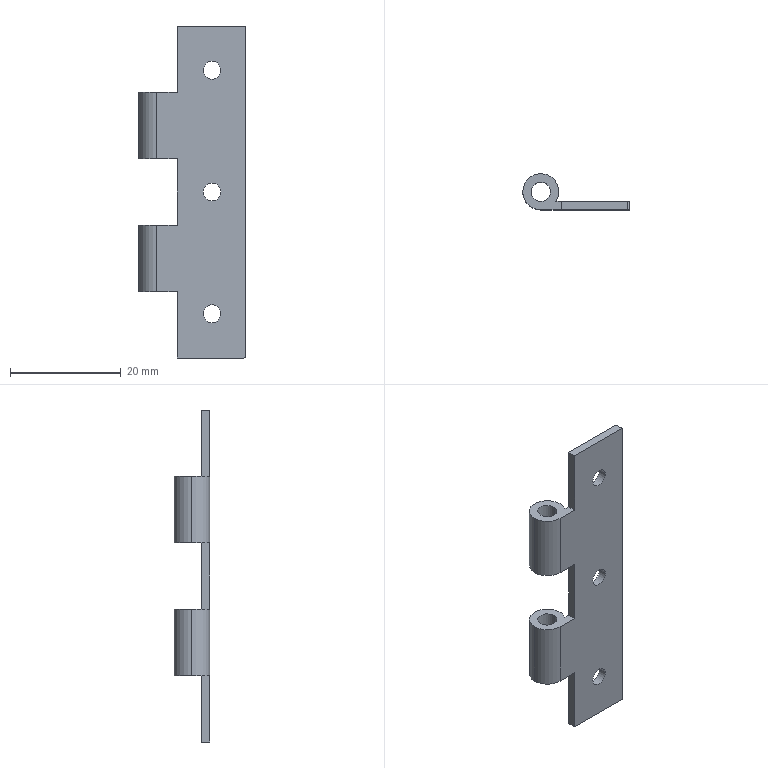Part | STEP file | Second B-1027-14 Pin B Part | 1 solid | 30 faces | box 19.25 x 6.5 x 60 mm | volume 1700 mm3 | cylinder 18 | plane 12 | commonest cylinder face diameters 3.2 x6 6.5 x6 3.5 x4 0.5 x2
STEP:
#1=CARTESIAN_POINT('',(-3.25,0.,18.));
#2=VERTEX_POINT('',#1);
#3=CARTESIAN_POINT('',(3.25,0.,18.));
#4=VERTEX_POINT('',#3);
#5=CARTESIAN_POINT('',(0.,0.,18.));
#6=DIRECTION('',(0.,0.,-1.));
#7=DIRECTION('',(-1.,0.,0.));
#8=AXIS2_PLACEMENT_3D('',#5,#6,#7);
#9=CIRCLE('',#8,3.25);
#10=EDGE_CURVE('',#2,#4,#9,.T.);
#11=ORIENTED_EDGE('',*,*,#10,.T.);
#12=CARTESIAN_POINT('',(3.25,0.,6.));
#13=VERTEX_POINT('',#12);
#14=CARTESIAN_POINT('',(3.25,0.,30.));
#15=DIRECTION('',(0.,0.,-1.));
#16=VECTOR('',#15,1000.);
#17=LINE('',#14,#16);
#18=EDGE_CURVE('',#4,#13,#17,.T.);
#19=ORIENTED_EDGE('',*,*,#18,.T.);
#20=CARTESIAN_POINT('',(-3.25,0.,6.));
#21=VERTEX_POINT('',#20);
#22=CARTESIAN_POINT('',(0.,0.,6.));
#23=DIRECTION('',(0.,0.,1.));
#24=DIRECTION('',(-1.,0.,0.));
#25=AXIS2_PLACEMENT_3D('',#22,#23,#24);
#26=CIRCLE('',#25,3.25);
#27=EDGE_CURVE('',#13,#21,#26,.T.);
#28=ORIENTED_EDGE('',*,*,#27,.T.);
#29=CARTESIAN_POINT('',(-3.25,0.,30.));
#30=DIRECTION('',(0.,0.,-1.));
#31=VECTOR('',#30,1000.);
#32=LINE('',#29,#31);
#33=EDGE_CURVE('',#2,#21,#32,.T.);
#34=ORIENTED_EDGE('',*,*,#33,.F.);
#35=EDGE_LOOP('',(#11,#19,#28,#34));
#36=FACE_OUTER_BOUND('',#35,.T.);
#37=CARTESIAN_POINT('',(0.,0.,30.));
#38=DIRECTION('',(0.,0.,-1.));
#39=DIRECTION('',(-1.,0.,0.));
#40=AXIS2_PLACEMENT_3D('',#37,#38,#39);
#41=CYLINDRICAL_SURFACE('',#40,3.25);
#42=ADVANCED_FACE('',(#36),#41,.T.);
#43=CARTESIAN_POINT('',(0.,-3.25,18.));
#44=VERTEX_POINT('',#43);
#45=CARTESIAN_POINT('',(0.,0.,18.));
#46=DIRECTION('',(0.,0.,-1.));
#47=DIRECTION('',(-1.,0.,0.));
#48=AXIS2_PLACEMENT_3D('',#45,#46,#47);
#49=CIRCLE('',#48,3.25);
#50=EDGE_CURVE('',#44,#2,#49,.T.);
#51=ORIENTED_EDGE('',*,*,#50,.T.);
#52=ORIENTED_EDGE('',*,*,#33,.T.);
#53=CARTESIAN_POINT('',(0.,-3.25,6.));
#54=VERTEX_POINT('',#53);
#55=CARTESIAN_POINT('',(0.,0.,6.));
#56=DIRECTION('',(0.,0.,1.));
#57=DIRECTION('',(-1.,0.,0.));
#58=AXIS2_PLACEMENT_3D('',#55,#56,#57);
#59=CIRCLE('',#58,3.25);
#60=EDGE_CURVE('',#21,#54,#59,.T.);
#61=ORIENTED_EDGE('',*,*,#60,.T.);
#62=CARTESIAN_POINT('',(0.,-3.25,30.));
#63=DIRECTION('',(0.,0.,1.));
#64=VECTOR('',#63,1000.);
#65=LINE('',#62,#64);
#66=EDGE_CURVE('',#54,#44,#65,.T.);
#67=ORIENTED_EDGE('',*,*,#66,.T.);
#68=EDGE_LOOP('',(#51,#52,#61,#67));
#69=FACE_OUTER_BOUND('',#68,.T.);
#70=CARTESIAN_POINT('',(0.,0.,30.));
#71=DIRECTION('',(0.,0.,-1.));
#72=DIRECTION('',(-1.,0.,0.));
#73=AXIS2_PLACEMENT_3D('',#70,#71,#72);
#74=CYLINDRICAL_SURFACE('',#73,3.25);
#75=ADVANCED_FACE('',(#69),#74,.T.);
#76=CARTESIAN_POINT('',(-3.25,0.,-6.));
#77=VERTEX_POINT('',#76);
#78=CARTESIAN_POINT('',(3.25,0.,-6.));
#79=VERTEX_POINT('',#78);
#80=CARTESIAN_POINT('',(0.,0.,-6.));
#81=DIRECTION('',(0.,0.,-1.));
#82=DIRECTION('',(-1.,0.,0.));
#83=AXIS2_PLACEMENT_3D('',#80,#81,#82);
#84=CIRCLE('',#83,3.25);
#85=EDGE_CURVE('',#77,#79,#84,.T.);
#86=ORIENTED_EDGE('',*,*,#85,.T.);
#87=CARTESIAN_POINT('',(3.25,0.,-18.));
#88=VERTEX_POINT('',#87);
#89=CARTESIAN_POINT('',(3.25,0.,30.));
#90=DIRECTION('',(0.,0.,-1.));
#91=VECTOR('',#90,1000.);
#92=LINE('',#89,#91);
#93=EDGE_CURVE('',#79,#88,#92,.T.);
#94=ORIENTED_EDGE('',*,*,#93,.T.);
#95=CARTESIAN_POINT('',(-3.25,0.,-18.));
#96=VERTEX_POINT('',#95);
#97=CARTESIAN_POINT('',(0.,0.,-18.));
#98=DIRECTION('',(0.,0.,1.));
#99=DIRECTION('',(-1.,0.,0.));
#100=AXIS2_PLACEMENT_3D('',#97,#98,#99);
#101=CIRCLE('',#100,3.25);
#102=EDGE_CURVE('',#88,#96,#101,.T.);
#103=ORIENTED_EDGE('',*,*,#102,.T.);
#104=CARTESIAN_POINT('',(-3.25,0.,30.));
#105=DIRECTION('',(0.,0.,-1.));
#106=VECTOR('',#105,1000.);
#107=LINE('',#104,#106);
#108=EDGE_CURVE('',#77,#96,#107,.T.);
#109=ORIENTED_EDGE('',*,*,#108,.F.);
#110=EDGE_LOOP('',(#86,#94,#103,#109));
#111=FACE_OUTER_BOUND('',#110,.T.);
#112=CARTESIAN_POINT('',(0.,0.,30.));
#113=DIRECTION('',(0.,0.,-1.));
#114=DIRECTION('',(-1.,0.,0.));
#115=AXIS2_PLACEMENT_3D('',#112,#113,#114);
#116=CYLINDRICAL_SURFACE('',#115,3.25);
#117=ADVANCED_FACE('',(#111),#116,.T.);
#118=CARTESIAN_POINT('',(0.,-3.25,-6.));
#119=VERTEX_POINT('',#118);
#120=CARTESIAN_POINT('',(0.,0.,-6.));
#121=DIRECTION('',(0.,0.,-1.));
#122=DIRECTION('',(-1.,0.,0.));
#123=AXIS2_PLACEMENT_3D('',#120,#121,#122);
#124=CIRCLE('',#123,3.25);
#125=EDGE_CURVE('',#119,#77,#124,.T.);
#126=ORIENTED_EDGE('',*,*,#125,.T.);
#127=ORIENTED_EDGE('',*,*,#108,.T.);
#128=CARTESIAN_POINT('',(0.,-3.25,-18.));
#129=VERTEX_POINT('',#128);
#130=CARTESIAN_POINT('',(0.,0.,-18.));
#131=DIRECTION('',(0.,0.,1.));
#132=DIRECTION('',(-1.,0.,0.));
#133=AXIS2_PLACEMENT_3D('',#130,#131,#132);
#134=CIRCLE('',#133,3.25);
#135=EDGE_CURVE('',#96,#129,#134,.T.);
#136=ORIENTED_EDGE('',*,*,#135,.T.);
#137=CARTESIAN_POINT('',(0.,-3.25,30.));
#138=DIRECTION('',(0.,0.,1.));
#139=VECTOR('',#138,1000.);
#140=LINE('',#137,#139);
#141=EDGE_CURVE('',#129,#119,#140,.T.);
#142=ORIENTED_EDGE('',*,*,#141,.T.);
#143=EDGE_LOOP('',(#126,#127,#136,#142));
#144=FACE_OUTER_BOUND('',#143,.T.);
#145=CARTESIAN_POINT('',(0.,0.,30.));
#146=DIRECTION('',(0.,0.,-1.));
#147=DIRECTION('',(-1.,0.,0.));
#148=AXIS2_PLACEMENT_3D('',#145,#146,#147);
#149=CYLINDRICAL_SURFACE('',#148,3.25);
#150=ADVANCED_FACE('',(#144),#149,.T.);
#151=CARTESIAN_POINT('',(8.4,-3.25,-22.));
#152=VERTEX_POINT('',#151);
#153=CARTESIAN_POINT('',(11.6,-3.25,-22.));
#154=VERTEX_POINT('',#153);
#155=CARTESIAN_POINT('',(10.,-3.25,-22.));
#156=DIRECTION('',(0.,-1.,0.));
#157=DIRECTION('',(-1.,0.,0.));
#158=AXIS2_PLACEMENT_3D('',#155,#156,#157);
#159=CIRCLE('',#158,1.6);
#160=EDGE_CURVE('',#152,#154,#159,.T.);
#161=ORIENTED_EDGE('',*,*,#160,.T.);
#162=CARTESIAN_POINT('',(11.6,-1.75,-22.));
#163=VERTEX_POINT('',#162);
#164=CARTESIAN_POINT('',(11.6,-4.75,-22.));
#165=DIRECTION('',(0.,1.,0.));
#166=VECTOR('',#165,1000.);
#167=LINE('',#164,#166);
#168=EDGE_CURVE('',#154,#163,#167,.T.);
#169=ORIENTED_EDGE('',*,*,#168,.T.);
#170=CARTESIAN_POINT('',(8.4,-1.75,-22.));
#171=VERTEX_POINT('',#170);
#172=CARTESIAN_POINT('',(10.,-1.75,-22.));
#173=DIRECTION('',(0.,-1.,0.));
#174=DIRECTION('',(-1.,0.,0.));
#175=AXIS2_PLACEMENT_3D('',#172,#173,#174);
#176=CIRCLE('',#175,1.6);
#177=EDGE_CURVE('',#171,#163,#176,.T.);
#178=ORIENTED_EDGE('',*,*,#177,.F.);
#179=CARTESIAN_POINT('',(8.4,-4.75,-22.));
#180=DIRECTION('',(0.,1.,0.));
#181=VECTOR('',#180,1000.);
#182=LINE('',#179,#181);
#183=EDGE_CURVE('',#152,#171,#182,.T.);
#184=ORIENTED_EDGE('',*,*,#183,.F.);
#185=EDGE_LOOP('',(#161,#169,#178,#184));
#186=FACE_OUTER_BOUND('',#185,.T.);
#187=CARTESIAN_POINT('',(10.,-4.75,-22.));
#188=DIRECTION('',(0.,1.,0.));
#189=DIRECTION('',(-1.,0.,0.));
#190=AXIS2_PLACEMENT_3D('',#187,#188,#189);
#191=CYLINDRICAL_SURFACE('',#190,1.6);
#192=ADVANCED_FACE('',(#186),#191,.F.);
#193=CARTESIAN_POINT('',(8.4,-3.25,0.));
#194=VERTEX_POINT('',#193);
#195=CARTESIAN_POINT('',(11.6,-3.25,0.));
#196=VERTEX_POINT('',#195);
#197=CARTESIAN_POINT('',(10.,-3.25,0.));
#198=DIRECTION('',(0.,-1.,0.));
#199=DIRECTION('',(-1.,0.,0.));
#200=AXIS2_PLACEMENT_3D('',#197,#198,#199);
#201=CIRCLE('',#200,1.6);
#202=EDGE_CURVE('',#194,#196,#201,.T.);
#203=ORIENTED_EDGE('',*,*,#202,.T.);
#204=CARTESIAN_POINT('',(11.6,-1.75,0.));
#205=VERTEX_POINT('',#204);
#206=CARTESIAN_POINT('',(11.6,-4.75,0.));
#207=DIRECTION('',(0.,1.,0.));
#208=VECTOR('',#207,1000.);
#209=LINE('',#206,#208);
#210=EDGE_CURVE('',#196,#205,#209,.T.);
#211=ORIENTED_EDGE('',*,*,#210,.T.);
#212=CARTESIAN_POINT('',(8.4,-1.75,0.));
#213=VERTEX_POINT('',#212);
#214=CARTESIAN_POINT('',(10.,-1.75,0.));
#215=DIRECTION('',(0.,-1.,0.));
#216=DIRECTION('',(-1.,0.,0.));
#217=AXIS2_PLACEMENT_3D('',#214,#215,#216);
#218=CIRCLE('',#217,1.6);
#219=EDGE_CURVE('',#213,#205,#218,.T.);
#220=ORIENTED_EDGE('',*,*,#219,.F.);
#221=CARTESIAN_POINT('',(8.4,-4.75,0.));
#222=DIRECTION('',(0.,1.,0.));
#223=VECTOR('',#222,1000.);
#224=LINE('',#221,#223);
#225=EDGE_CURVE('',#194,#213,#224,.T.);
#226=ORIENTED_EDGE('',*,*,#225,.F.);
#227=EDGE_LOOP('',(#203,#211,#220,#226));
#228=FACE_OUTER_BOUND('',#227,.T.);
#229=CARTESIAN_POINT('',(10.,-4.75,0.));
#230=DIRECTION('',(0.,1.,0.));
#231=DIRECTION('',(-1.,0.,0.));
#232=AXIS2_PLACEMENT_3D('',#229,#230,#231);
#233=CYLINDRICAL_SURFACE('',#232,1.6);
#234=ADVANCED_FACE('',(#228),#233,.F.);
#235=CARTESIAN_POINT('',(8.4,-3.25,22.));
#236=VERTEX_POINT('',#235);
#237=CARTESIAN_POINT('',(11.6,-3.25,22.));
#238=VERTEX_POINT('',#237);
#239=CARTESIAN_POINT('',(10.,-3.25,22.));
#240=DIRECTION('',(0.,-1.,0.));
#241=DIRECTION('',(-1.,0.,0.));
#242=AXIS2_PLACEMENT_3D('',#239,#240,#241);
#243=CIRCLE('',#242,1.6);
#244=EDGE_CURVE('',#236,#238,#243,.T.);
#245=ORIENTED_EDGE('',*,*,#244,.T.);
#246=CARTESIAN_POINT('',(11.6,-1.75,22.));
#247=VERTEX_POINT('',#246);
#248=CARTESIAN_POINT('',(11.6,-4.75,22.));
#249=DIRECTION('',(0.,1.,0.));
#250=VECTOR('',#249,1000.);
#251=LINE('',#248,#250);
#252=EDGE_CURVE('',#238,#247,#251,.T.);
#253=ORIENTED_EDGE('',*,*,#252,.T.);
#254=CARTESIAN_POINT('',(8.4,-1.75,22.));
#255=VERTEX_POINT('',#254);
#256=CARTESIAN_POINT('',(10.,-1.75,22.));
#257=DIRECTION('',(0.,-1.,0.));
#258=DIRECTION('',(-1.,0.,0.));
#259=AXIS2_PLACEMENT_3D('',#256,#257,#258);
#260=CIRCLE('',#259,1.6);
#261=EDGE_CURVE('',#255,#247,#260,.T.);
#262=ORIENTED_EDGE('',*,*,#261,.F.);
#263=CARTESIAN_POINT('',(8.4,-4.75,22.));
#264=DIRECTION('',(0.,1.,0.));
#265=VECTOR('',#264,1000.);
#266=LINE('',#263,#265);
#267=EDGE_CURVE('',#236,#255,#266,.T.);
#268=ORIENTED_EDGE('',*,*,#267,.F.);
#269=EDGE_LOOP('',(#245,#253,#262,#268));
#270=FACE_OUTER_BOUND('',#269,.T.);
#271=CARTESIAN_POINT('',(10.,-4.75,22.));
#272=DIRECTION('',(0.,1.,0.));
#273=DIRECTION('',(-1.,0.,0.));
#274=AXIS2_PLACEMENT_3D('',#271,#272,#273);
#275=CYLINDRICAL_SURFACE('',#274,1.6);
#276=ADVANCED_FACE('',(#270),#275,.F.);
#277=CARTESIAN_POINT('',(-1.75,0.,18.));
#278=VERTEX_POINT('',#277);
#279=CARTESIAN_POINT('',(1.75,0.,18.));
#280=VERTEX_POINT('',#279);
#281=CARTESIAN_POINT('',(0.,0.,18.));
#282=DIRECTION('',(0.,0.,1.));
#283=DIRECTION('',(-1.,0.,0.));
#284=AXIS2_PLACEMENT_3D('',#281,#282,#283);
#285=CIRCLE('',#284,1.75);
#286=EDGE_CURVE('',#278,#280,#285,.T.);
#287=ORIENTED_EDGE('',*,*,#286,.T.);
#288=CARTESIAN_POINT('',(1.75,0.,6.));
#289=VERTEX_POINT('',#288);
#290=CARTESIAN_POINT('',(1.75,0.,30.));
#291=DIRECTION('',(0.,0.,-1.));
#292=VECTOR('',#291,1000.);
#293=LINE('',#290,#292);
#294=EDGE_CURVE('',#280,#289,#293,.T.);
#295=ORIENTED_EDGE('',*,*,#294,.T.);
#296=CARTESIAN_POINT('',(-1.75,0.,6.));
#297=VERTEX_POINT('',#296);
#298=CARTESIAN_POINT('',(0.,0.,6.));
#299=DIRECTION('',(0.,0.,-1.));
#300=DIRECTION('',(-1.,0.,0.));
#301=AXIS2_PLACEMENT_3D('',#298,#299,#300);
#302=CIRCLE('',#301,1.75);
#303=EDGE_CURVE('',#289,#297,#302,.T.);
#304=ORIENTED_EDGE('',*,*,#303,.T.);
#305=CARTESIAN_POINT('',(-1.75,0.,30.));
#306=DIRECTION('',(0.,0.,-1.));
#307=VECTOR('',#306,1000.);
#308=LINE('',#305,#307);
#309=EDGE_CURVE('',#278,#297,#308,.T.);
#310=ORIENTED_EDGE('',*,*,#309,.F.);
#311=EDGE_LOOP('',(#287,#295,#304,#310));
#312=FACE_OUTER_BOUND('',#311,.T.);
#313=CARTESIAN_POINT('',(0.,0.,30.));
#314=DIRECTION('',(0.,0.,-1.));
#315=DIRECTION('',(-1.,0.,0.));
#316=AXIS2_PLACEMENT_3D('',#313,#314,#315);
#317=CYLINDRICAL_SURFACE('',#316,1.75);
#318=ADVANCED_FACE('',(#312),#317,.F.);
#319=CARTESIAN_POINT('',(-1.75,0.,-6.));
#320=VERTEX_POINT('',#319);
#321=CARTESIAN_POINT('',(1.75,0.,-6.));
#322=VERTEX_POINT('',#321);
#323=CARTESIAN_POINT('',(0.,0.,-6.));
#324=DIRECTION('',(0.,0.,1.));
#325=DIRECTION('',(-1.,0.,0.));
#326=AXIS2_PLACEMENT_3D('',#323,#324,#325);
#327=CIRCLE('',#326,1.75);
#328=EDGE_CURVE('',#320,#322,#327,.T.);
#329=ORIENTED_EDGE('',*,*,#328,.T.);
#330=CARTESIAN_POINT('',(1.75,0.,-18.));
#331=VERTEX_POINT('',#330);
#332=CARTESIAN_POINT('',(1.75,0.,30.));
#333=DIRECTION('',(0.,0.,-1.));
#334=VECTOR('',#333,1000.);
#335=LINE('',#332,#334);
#336=EDGE_CURVE('',#322,#331,#335,.T.);
#337=ORIENTED_EDGE('',*,*,#336,.T.);
#338=CARTESIAN_POINT('',(-1.75,0.,-18.));
#339=VERTEX_POINT('',#338);
#340=CARTESIAN_POINT('',(0.,0.,-18.));
#341=DIRECTION('',(0.,0.,-1.));
#342=DIRECTION('',(-1.,0.,0.));
#343=AXIS2_PLACEMENT_3D('',#340,#341,#342);
#344=CIRCLE('',#343,1.75);
#345=EDGE_CURVE('',#331,#339,#344,.T.);
#346=ORIENTED_EDGE('',*,*,#345,.T.);
#347=CARTESIAN_POINT('',(-1.75,0.,30.));
#348=DIRECTION('',(0.,0.,-1.));
#349=VECTOR('',#348,1000.);
#350=LINE('',#347,#349);
#351=EDGE_CURVE('',#320,#339,#350,.T.);
#352=ORIENTED_EDGE('',*,*,#351,.F.);
#353=EDGE_LOOP('',(#329,#337,#346,#352));
#354=FACE_OUTER_BOUND('',#353,.T.);
#355=CARTESIAN_POINT('',(0.,0.,30.));
#356=DIRECTION('',(0.,0.,-1.));
#357=DIRECTION('',(-1.,0.,0.));
#358=AXIS2_PLACEMENT_3D('',#355,#356,#357);
#359=CYLINDRICAL_SURFACE('',#358,1.75);
#360=ADVANCED_FACE('',(#354),#359,.F.);
#361=CARTESIAN_POINT('',(15.75,-3.25,30.));
#362=VERTEX_POINT('',#361);
#363=CARTESIAN_POINT('',(16.,-3.25,29.75));
#364=VERTEX_POINT('',#363);
#365=CARTESIAN_POINT('',(15.75,-3.25,29.75));
#366=DIRECTION('',(0.,1.,0.));
#367=DIRECTION('',(0.,0.,-1.));
#368=AXIS2_PLACEMENT_3D('',#365,#366,#367);
#369=CIRCLE('',#368,0.25);
#370=EDGE_CURVE('',#362,#364,#369,.T.);
#371=ORIENTED_EDGE('',*,*,#370,.F.);
#372=CARTESIAN_POINT('',(3.7,-3.25,30.));
#373=VERTEX_POINT('',#372);
#374=CARTESIAN_POINT('',(0.,-3.25,30.));
#375=DIRECTION('',(1.,0.,0.));
#376=VECTOR('',#375,1000.);
#377=LINE('',#374,#376);
#378=EDGE_CURVE('',#373,#362,#377,.T.);
#379=ORIENTED_EDGE('',*,*,#378,.F.);
#380=CARTESIAN_POINT('',(3.7,-3.25,18.));
#381=VERTEX_POINT('',#380);
#382=CARTESIAN_POINT('',(3.7,-3.25,30.));
#383=DIRECTION('',(0.,0.,1.));
#384=VECTOR('',#383,1000.);
#385=LINE('',#382,#384);
#386=EDGE_CURVE('',#381,#373,#385,.T.);
#387=ORIENTED_EDGE('',*,*,#386,.F.);
#388=CARTESIAN_POINT('',(0.,-3.25,18.));
#389=DIRECTION('',(1.,0.,0.));
#390=VECTOR('',#389,1000.);
#391=LINE('',#388,#390);
#392=EDGE_CURVE('',#44,#381,#391,.T.);
#393=ORIENTED_EDGE('',*,*,#392,.F.);
#394=ORIENTED_EDGE('',*,*,#66,.F.);
#395=CARTESIAN_POINT('',(3.7,-3.25,6.));
#396=VERTEX_POINT('',#395);
#397=CARTESIAN_POINT('',(0.,-3.25,6.));
#398=DIRECTION('',(-1.,0.,0.));
#399=VECTOR('',#398,1000.);
#400=LINE('',#397,#399);
#401=EDGE_CURVE('',#396,#54,#400,.T.);
#402=ORIENTED_EDGE('',*,*,#401,.F.);
#403=CARTESIAN_POINT('',(3.7,-3.25,-6.));
#404=VERTEX_POINT('',#403);
#405=CARTESIAN_POINT('',(3.7,-3.25,30.));
#406=DIRECTION('',(0.,0.,1.));
#407=VECTOR('',#406,1000.);
#408=LINE('',#405,#407);
#409=EDGE_CURVE('',#404,#396,#408,.T.);
#410=ORIENTED_EDGE('',*,*,#409,.F.);
#411=CARTESIAN_POINT('',(0.,-3.25,-6.));
#412=DIRECTION('',(1.,0.,0.));
#413=VECTOR('',#412,1000.);
#414=LINE('',#411,#413);
#415=EDGE_CURVE('',#119,#404,#414,.T.);
#416=ORIENTED_EDGE('',*,*,#415,.F.);
#417=ORIENTED_EDGE('',*,*,#141,.F.);
#418=CARTESIAN_POINT('',(3.7,-3.25,-18.));
#419=VERTEX_POINT('',#418);
#420=CARTESIAN_POINT('',(0.,-3.25,-18.));
#421=DIRECTION('',(-1.,0.,0.));
#422=VECTOR('',#421,1000.);
#423=LINE('',#420,#422);
#424=EDGE_CURVE('',#419,#129,#423,.T.);
#425=ORIENTED_EDGE('',*,*,#424,.F.);
#426=CARTESIAN_POINT('',(3.7,-3.25,-30.));
#427=VERTEX_POINT('',#426);
#428=CARTESIAN_POINT('',(3.7,-3.25,30.));
#429=DIRECTION('',(0.,0.,1.));
#430=VECTOR('',#429,1000.);
#431=LINE('',#428,#430);
#432=EDGE_CURVE('',#427,#419,#431,.T.);
#433=ORIENTED_EDGE('',*,*,#432,.F.);
#434=CARTESIAN_POINT('',(15.75,-3.25,-30.));
#435=VERTEX_POINT('',#434);
#436=CARTESIAN_POINT('',(0.,-3.25,-30.));
#437=DIRECTION('',(-1.,0.,0.));
#438=VECTOR('',#437,1000.);
#439=LINE('',#436,#438);
#440=EDGE_CURVE('',#435,#427,#439,.T.);
#441=ORIENTED_EDGE('',*,*,#440,.F.);
#442=CARTESIAN_POINT('',(16.,-3.25,-29.75));
#443=VERTEX_POINT('',#442);
#444=CARTESIAN_POINT('',(15.75,-3.25,-29.75));
#445=DIRECTION('',(0.,1.,0.));
#446=DIRECTION('',(0.,0.,1.));
#447=AXIS2_PLACEMENT_3D('',#444,#445,#446);
#448=CIRCLE('',#447,0.25);
#449=EDGE_CURVE('',#443,#435,#448,.T.);
#450=ORIENTED_EDGE('',*,*,#449,.F.);
#451=CARTESIAN_POINT('',(16.,-3.25,30.));
#452=DIRECTION('',(0.,0.,-1.));
#453=VECTOR('',#452,1000.);
#454=LINE('',#451,#453);
#455=EDGE_CURVE('',#364,#443,#454,.T.);
#456=ORIENTED_EDGE('',*,*,#455,.F.);
#457=EDGE_LOOP('',(#371,#379,#387,#393,#394,#402,#410,#416,#417,#425,#433,#441,#450,#456));
#458=FACE_OUTER_BOUND('',#457,.T.);
#459=ORIENTED_EDGE('',*,*,#160,.F.);
#460=CARTESIAN_POINT('',(10.,-3.25,-22.));
#461=DIRECTION('',(0.,-1.,0.));
#462=DIRECTION('',(-1.,0.,0.));
#463=AXIS2_PLACEMENT_3D('',#460,#461,#462);
#464=CIRCLE('',#463,1.6);
#465=EDGE_CURVE('',#154,#152,#464,.T.);
#466=ORIENTED_EDGE('',*,*,#465,.F.);
#467=EDGE_LOOP('',(#459,#466));
#468=FACE_BOUND('',#467,.T.);
#469=ORIENTED_EDGE('',*,*,#202,.F.);
#470=CARTESIAN_POINT('',(10.,-3.25,0.));
#471=DIRECTION('',(0.,-1.,0.));
#472=DIRECTION('',(-1.,0.,0.));
#473=AXIS2_PLACEMENT_3D('',#470,#471,#472);
#474=CIRCLE('',#473,1.6);
#475=EDGE_CURVE('',#196,#194,#474,.T.);
#476=ORIENTED_EDGE('',*,*,#475,.F.);
#477=EDGE_LOOP('',(#469,#476));
#478=FACE_BOUND('',#477,.T.);
#479=ORIENTED_EDGE('',*,*,#244,.F.);
#480=CARTESIAN_POINT('',(10.,-3.25,22.));
#481=DIRECTION('',(0.,-1.,0.));
#482=DIRECTION('',(-1.,0.,0.));
#483=AXIS2_PLACEMENT_3D('',#480,#481,#482);
#484=CIRCLE('',#483,1.6);
#485=EDGE_CURVE('',#238,#236,#484,.T.);
#486=ORIENTED_EDGE('',*,*,#485,.F.);
#487=EDGE_LOOP('',(#479,#486));
#488=FACE_BOUND('',#487,.T.);
#489=CARTESIAN_POINT('',(0.,-3.25,30.));
#490=DIRECTION('',(0.,1.,0.));
#491=DIRECTION('',(-1.,0.,0.));
#492=AXIS2_PLACEMENT_3D('',#489,#490,#491);
#493=PLANE('',#492);
#494=ADVANCED_FACE('',(#458,#468,#478,#488),#493,.F.);
#495=CARTESIAN_POINT('',(16.,-1.75,29.75));
#496=VERTEX_POINT('',#495);
#497=CARTESIAN_POINT('',(16.,-3.25,29.75));
#498=DIRECTION('',(0.,1.,0.));
#499=VECTOR('',#498,1000.);
#500=LINE('',#497,#499);
#501=EDGE_CURVE('',#364,#496,#500,.T.);
#502=ORIENTED_EDGE('',*,*,#501,.F.);
#503=ORIENTED_EDGE('',*,*,#455,.T.);
#504=CARTESIAN_POINT('',(16.,-1.75,-29.75));
#505=VERTEX_POINT('',#504);
#506=CARTESIAN_POINT('',(16.,-3.25,-29.75));
#507=DIRECTION('',(0.,-1.,0.));
#508=VECTOR('',#507,1000.);
#509=LINE('',#506,#508);
#510=EDGE_CURVE('',#505,#443,#509,.T.);
#511=ORIENTED_EDGE('',*,*,#510,.F.);
#512=CARTESIAN_POINT('',(16.,-1.75,30.));
#513=DIRECTION('',(0.,0.,-1.));
#514=VECTOR('',#513,1000.);
#515=LINE('',#512,#514);
#516=EDGE_CURVE('',#496,#505,#515,.T.);
#517=ORIENTED_EDGE('',*,*,#516,.F.);
#518=EDGE_LOOP('',(#502,#503,#511,#517));
#519=FACE_OUTER_BOUND('',#518,.T.);
#520=CARTESIAN_POINT('',(16.,-3.25,30.));
#521=DIRECTION('',(-1.,0.,0.));
#522=DIRECTION('',(0.,0.,1.));
#523=AXIS2_PLACEMENT_3D('',#520,#521,#522);
#524=PLANE('',#523);
#525=ADVANCED_FACE('',(#519),#524,.F.);
#526=CARTESIAN_POINT('',(15.75,-1.75,30.));
#527=VERTEX_POINT('',#526);
#528=CARTESIAN_POINT('',(3.7,-1.75,30.));
#529=VERTEX_POINT('',#528);
#530=CARTESIAN_POINT('',(0.,-1.75,30.));
#531=DIRECTION('',(-1.,0.,0.));
#532=VECTOR('',#531,1000.);
#533=LINE('',#530,#532);
#534=EDGE_CURVE('',#527,#529,#533,.T.);
#535=ORIENTED_EDGE('',*,*,#534,.T.);
#536=CARTESIAN_POINT('',(3.7,0.,30.));
#537=DIRECTION('',(0.,-1.,0.));
#538=VECTOR('',#537,1000.);
#539=LINE('',#536,#538);
#540=EDGE_CURVE('',#529,#373,#539,.T.);
#541=ORIENTED_EDGE('',*,*,#540,.T.);
#542=ORIENTED_EDGE('',*,*,#378,.T.);
#543=CARTESIAN_POINT('',(15.75,0.,30.));
#544=DIRECTION('',(0.,1.,0.));
#545=VECTOR('',#544,1000.);
#546=LINE('',#543,#545);
#547=EDGE_CURVE('',#362,#527,#546,.T.);
#548=ORIENTED_EDGE('',*,*,#547,.T.);
#549=EDGE_LOOP('',(#535,#541,#542,#548));
#550=FACE_OUTER_BOUND('',#549,.T.);
#551=CARTESIAN_POINT('',(0.,0.,30.));
#552=DIRECTION('',(0.,0.,1.));
#553=DIRECTION('',(1.,0.,0.));
#554=AXIS2_PLACEMENT_3D('',#551,#552,#553);
#555=PLANE('',#554);
#556=ADVANCED_FACE('',(#550),#555,.T.);
#557=CARTESIAN_POINT('',(3.7,-1.75,18.));
#558=VERTEX_POINT('',#557);
#559=CARTESIAN_POINT('',(3.7,-1.75,30.));
#560=DIRECTION('',(0.,0.,1.));
#561=VECTOR('',#560,1000.);
#562=LINE('',#559,#561);
#563=EDGE_CURVE('',#558,#529,#562,.T.);
#564=ORIENTED_EDGE('',*,*,#563,.F.);
#565=CARTESIAN_POINT('',(3.7,-31.75,18.));
#566=DIRECTION('',(0.,1.,0.));
#567=VECTOR('',#566,1000.);
#568=LINE('',#565,#567);
#569=EDGE_CURVE('',#381,#558,#568,.T.);
#570=ORIENTED_EDGE('',*,*,#569,.F.);
#571=ORIENTED_EDGE('',*,*,#386,.T.);
#572=ORIENTED_EDGE('',*,*,#540,.F.);
#573=EDGE_LOOP('',(#564,#570,#571,#572));
#574=FACE_OUTER_BOUND('',#573,.T.);
#575=CARTESIAN_POINT('',(3.7,-31.75,30.));
#576=DIRECTION('',(1.,0.,0.));
#577=DIRECTION('',(0.,1.,0.));
#578=AXIS2_PLACEMENT_3D('',#575,#576,#577);
#579=PLANE('',#578);
#580=ADVANCED_FACE('',(#574),#579,.F.);
#581=CARTESIAN_POINT('',(2.739,-1.75,18.));
#582=VERTEX_POINT('',#581);
#583=CARTESIAN_POINT('',(-3.25,-1.75,18.));
#584=DIRECTION('',(1.,0.,0.));
#585=VECTOR('',#584,1000.);
#586=LINE('',#583,#585);
#587=EDGE_CURVE('',#582,#558,#586,.T.);
#588=ORIENTED_EDGE('',*,*,#587,.F.);
#589=CARTESIAN_POINT('',(0.,0.,18.));
#590=DIRECTION('',(0.,0.,-1.));
#591=DIRECTION('',(-1.,0.,0.));
#592=AXIS2_PLACEMENT_3D('',#589,#590,#591);
#593=CIRCLE('',#592,3.25);
#594=EDGE_CURVE('',#4,#582,#593,.T.);
#595=ORIENTED_EDGE('',*,*,#594,.F.);
#596=ORIENTED_EDGE('',*,*,#10,.F.);
#597=ORIENTED_EDGE('',*,*,#50,.F.);
#598=ORIENTED_EDGE('',*,*,#392,.T.);
#599=ORIENTED_EDGE('',*,*,#569,.T.);
#600=EDGE_LOOP('',(#588,#595,#596,#597,#598,#599));
#601=FACE_OUTER_BOUND('',#600,.T.);
#602=ORIENTED_EDGE('',*,*,#286,.F.);
#603=CARTESIAN_POINT('',(0.,0.,18.));
#604=DIRECTION('',(0.,0.,1.));
#605=DIRECTION('',(-1.,0.,0.));
#606=AXIS2_PLACEMENT_3D('',#603,#604,#605);
#607=CIRCLE('',#606,1.75);
#608=EDGE_CURVE('',#280,#278,#607,.T.);
#609=ORIENTED_EDGE('',*,*,#608,.F.);
#610=EDGE_LOOP('',(#602,#609));
#611=FACE_BOUND('',#610,.T.);
#612=CARTESIAN_POINT('',(-3.25,-31.75,18.));
#613=DIRECTION('',(0.,0.,-1.));
#614=DIRECTION('',(-1.,0.,0.));
#615=AXIS2_PLACEMENT_3D('',#612,#613,#614);
#616=PLANE('',#615);
#617=ADVANCED_FACE('',(#601,#611),#616,.F.);
#618=ORIENTED_EDGE('',*,*,#18,.F.);
#619=ORIENTED_EDGE('',*,*,#594,.T.);
#620=CARTESIAN_POINT('',(2.739,-1.75,6.));
#621=VERTEX_POINT('',#620);
#622=CARTESIAN_POINT('',(2.739,-1.75,30.));
#623=DIRECTION('',(0.,0.,-1.));
#624=VECTOR('',#623,1000.);
#625=LINE('',#622,#624);
#626=EDGE_CURVE('',#582,#621,#625,.T.);
#627=ORIENTED_EDGE('',*,*,#626,.T.);
#628=CARTESIAN_POINT('',(0.,0.,6.));
#629=DIRECTION('',(0.,0.,1.));
#630=DIRECTION('',(-1.,0.,0.));
#631=AXIS2_PLACEMENT_3D('',#628,#629,#630);
#632=CIRCLE('',#631,3.25);
#633=EDGE_CURVE('',#621,#13,#632,.T.);
#634=ORIENTED_EDGE('',*,*,#633,.T.);
#635=EDGE_LOOP('',(#618,#619,#627,#634));
#636=FACE_OUTER_BOUND('',#635,.T.);
#637=CARTESIAN_POINT('',(0.,0.,30.));
#638=DIRECTION('',(0.,0.,-1.));
#639=DIRECTION('',(-1.,0.,0.));
#640=AXIS2_PLACEMENT_3D('',#637,#638,#639);
#641=CYLINDRICAL_SURFACE('',#640,3.25);
#642=ADVANCED_FACE('',(#636),#641,.T.);
#643=CARTESIAN_POINT('',(3.7,-1.75,6.));
#644=VERTEX_POINT('',#643);
#645=CARTESIAN_POINT('',(-3.25,-1.75,6.));
#646=DIRECTION('',(-1.,0.,0.));
#647=VECTOR('',#646,1000.);
#648=LINE('',#645,#647);
#649=EDGE_CURVE('',#644,#621,#648,.T.);
#650=ORIENTED_EDGE('',*,*,#649,.F.);
#651=CARTESIAN_POINT('',(3.7,-31.75,6.));
#652=DIRECTION('',(0.,1.,0.));
#653=VECTOR('',#652,1000.);
#654=LINE('',#651,#653);
#655=EDGE_CURVE('',#396,#644,#654,.T.);
#656=ORIENTED_EDGE('',*,*,#655,.F.);
#657=ORIENTED_EDGE('',*,*,#401,.T.);
#658=ORIENTED_EDGE('',*,*,#60,.F.);
#659=ORIENTED_EDGE('',*,*,#27,.F.);
#660=ORIENTED_EDGE('',*,*,#633,.F.);
#661=EDGE_LOOP('',(#650,#656,#657,#658,#659,#660));
#662=FACE_OUTER_BOUND('',#661,.T.);
#663=CARTESIAN_POINT('',(0.,0.,6.));
#664=DIRECTION('',(0.,0.,-1.));
#665=DIRECTION('',(-1.,0.,0.));
#666=AXIS2_PLACEMENT_3D('',#663,#664,#665);
#667=CIRCLE('',#666,1.75);
#668=EDGE_CURVE('',#297,#289,#667,.T.);
#669=ORIENTED_EDGE('',*,*,#668,.F.);
#670=ORIENTED_EDGE('',*,*,#303,.F.);
#671=EDGE_LOOP('',(#669,#670));
#672=FACE_BOUND('',#671,.T.);
#673=CARTESIAN_POINT('',(-3.25,-31.75,6.));
#674=DIRECTION('',(0.,0.,1.));
#675=DIRECTION('',(1.,0.,0.));
#676=AXIS2_PLACEMENT_3D('',#673,#674,#675);
#677=PLANE('',#676);
#678=ADVANCED_FACE('',(#662,#672),#677,.F.);
#679=CARTESIAN_POINT('',(3.7,-1.75,-6.));
#680=VERTEX_POINT('',#679);
#681=CARTESIAN_POINT('',(3.7,-1.75,-6.));
#682=DIRECTION('',(0.,0.,1.));
#683=VECTOR('',#682,1000.);
#684=LINE('',#681,#683);
#685=EDGE_CURVE('',#680,#644,#684,.T.);
#686=ORIENTED_EDGE('',*,*,#685,.F.);
#687=CARTESIAN_POINT('',(3.7,-31.75,-6.));
#688=DIRECTION('',(0.,1.,0.));
#689=VECTOR('',#688,1000.);
#690=LINE('',#687,#689);
#691=EDGE_CURVE('',#404,#680,#690,.T.);
#692=ORIENTED_EDGE('',*,*,#691,.F.);
#693=ORIENTED_EDGE('',*,*,#409,.T.);
#694=ORIENTED_EDGE('',*,*,#655,.T.);
#695=EDGE_LOOP('',(#686,#692,#693,#694));
#696=FACE_OUTER_BOUND('',#695,.T.);
#697=CARTESIAN_POINT('',(3.7,-31.75,-6.));
#698=DIRECTION('',(1.,0.,0.));
#699=DIRECTION('',(0.,0.,-1.));
#700=AXIS2_PLACEMENT_3D('',#697,#698,#699);
#701=PLANE('',#700);
#702=ADVANCED_FACE('',(#696),#701,.F.);
#703=CARTESIAN_POINT('',(2.739,-1.75,-6.));
#704=VERTEX_POINT('',#703);
#705=CARTESIAN_POINT('',(-3.25,-1.75,-6.));
#706=DIRECTION('',(1.,0.,0.));
#707=VECTOR('',#706,1000.);
#708=LINE('',#705,#707);
#709=EDGE_CURVE('',#704,#680,#708,.T.);
#710=ORIENTED_EDGE('',*,*,#709,.F.);
#711=CARTESIAN_POINT('',(0.,0.,-6.));
#712=DIRECTION('',(0.,0.,-1.));
#713=DIRECTION('',(-1.,0.,0.));
#714=AXIS2_PLACEMENT_3D('',#711,#712,#713);
#715=CIRCLE('',#714,3.25);
#716=EDGE_CURVE('',#79,#704,#715,.T.);
#717=ORIENTED_EDGE('',*,*,#716,.F.);
#718=ORIENTED_EDGE('',*,*,#85,.F.);
#719=ORIENTED_EDGE('',*,*,#125,.F.);
#720=ORIENTED_EDGE('',*,*,#415,.T.);
#721=ORIENTED_EDGE('',*,*,#691,.T.);
#722=EDGE_LOOP('',(#710,#717,#718,#719,#720,#721));
#723=FACE_OUTER_BOUND('',#722,.T.);
#724=ORIENTED_EDGE('',*,*,#328,.F.);
#725=CARTESIAN_POINT('',(0.,0.,-6.));
#726=DIRECTION('',(0.,0.,1.));
#727=DIRECTION('',(-1.,0.,0.));
#728=AXIS2_PLACEMENT_3D('',#725,#726,#727);
#729=CIRCLE('',#728,1.75);
#730=EDGE_CURVE('',#322,#320,#729,.T.);
#731=ORIENTED_EDGE('',*,*,#730,.F.);
#732=EDGE_LOOP('',(#724,#731));
#733=FACE_BOUND('',#732,.T.);
#734=CARTESIAN_POINT('',(-3.25,-31.75,-6.));
#735=DIRECTION('',(0.,0.,-1.));
#736=DIRECTION('',(-1.,0.,0.));
#737=AXIS2_PLACEMENT_3D('',#734,#735,#736);
#738=PLANE('',#737);
#739=ADVANCED_FACE('',(#723,#733),#738,.F.);
#740=ORIENTED_EDGE('',*,*,#93,.F.);
#741=ORIENTED_EDGE('',*,*,#716,.T.);
#742=CARTESIAN_POINT('',(2.739,-1.75,-18.));
#743=VERTEX_POINT('',#742);
#744=CARTESIAN_POINT('',(2.739,-1.75,30.));
#745=DIRECTION('',(0.,0.,-1.));
#746=VECTOR('',#745,1000.);
#747=LINE('',#744,#746);
#748=EDGE_CURVE('',#704,#743,#747,.T.);
#749=ORIENTED_EDGE('',*,*,#748,.T.);
#750=CARTESIAN_POINT('',(0.,0.,-18.));
#751=DIRECTION('',(0.,0.,1.));
#752=DIRECTION('',(-1.,0.,0.));
#753=AXIS2_PLACEMENT_3D('',#750,#751,#752);
#754=CIRCLE('',#753,3.25);
#755=EDGE_CURVE('',#743,#88,#754,.T.);
#756=ORIENTED_EDGE('',*,*,#755,.T.);
#757=EDGE_LOOP('',(#740,#741,#749,#756));
#758=FACE_OUTER_BOUND('',#757,.T.);
#759=CARTESIAN_POINT('',(0.,0.,30.));
#760=DIRECTION('',(0.,0.,-1.));
#761=DIRECTION('',(-1.,0.,0.));
#762=AXIS2_PLACEMENT_3D('',#759,#760,#761);
#763=CYLINDRICAL_SURFACE('',#762,3.25);
#764=ADVANCED_FACE('',(#758),#763,.T.);
#765=CARTESIAN_POINT('',(3.7,-1.75,-18.));
#766=VERTEX_POINT('',#765);
#767=CARTESIAN_POINT('',(-3.25,-1.75,-18.));
#768=DIRECTION('',(-1.,0.,0.));
#769=VECTOR('',#768,1000.);
#770=LINE('',#767,#769);
#771=EDGE_CURVE('',#766,#743,#770,.T.);
#772=ORIENTED_EDGE('',*,*,#771,.F.);
#773=CARTESIAN_POINT('',(3.7,-31.75,-18.));
#774=DIRECTION('',(0.,1.,0.));
#775=VECTOR('',#774,1000.);
#776=LINE('',#773,#775);
#777=EDGE_CURVE('',#419,#766,#776,.T.);
#778=ORIENTED_EDGE('',*,*,#777,.F.);
#779=ORIENTED_EDGE('',*,*,#424,.T.);
#780=ORIENTED_EDGE('',*,*,#135,.F.);
#781=ORIENTED_EDGE('',*,*,#102,.F.);
#782=ORIENTED_EDGE('',*,*,#755,.F.);
#783=EDGE_LOOP('',(#772,#778,#779,#780,#781,#782));
#784=FACE_OUTER_BOUND('',#783,.T.);
#785=CARTESIAN_POINT('',(0.,0.,-18.));
#786=DIRECTION('',(0.,0.,-1.));
#787=DIRECTION('',(-1.,0.,0.));
#788=AXIS2_PLACEMENT_3D('',#785,#786,#787);
#789=CIRCLE('',#788,1.75);
#790=EDGE_CURVE('',#339,#331,#789,.T.);
#791=ORIENTED_EDGE('',*,*,#790,.F.);
#792=ORIENTED_EDGE('',*,*,#345,.F.);
#793=EDGE_LOOP('',(#791,#792));
#794=FACE_BOUND('',#793,.T.);
#795=CARTESIAN_POINT('',(-3.25,-31.75,-18.));
#796=DIRECTION('',(0.,0.,1.));
#797=DIRECTION('',(1.,0.,0.));
#798=AXIS2_PLACEMENT_3D('',#795,#796,#797);
#799=PLANE('',#798);
#800=ADVANCED_FACE('',(#784,#794),#799,.F.);
#801=CARTESIAN_POINT('',(3.7,-1.75,-30.));
#802=VERTEX_POINT('',#801);
#803=CARTESIAN_POINT('',(3.7,-1.75,-30.));
#804=DIRECTION('',(0.,0.,1.));
#805=VECTOR('',#804,1000.);
#806=LINE('',#803,#805);
#807=EDGE_CURVE('',#802,#766,#806,.T.);
#808=ORIENTED_EDGE('',*,*,#807,.F.);
#809=CARTESIAN_POINT('',(3.7,-31.75,-30.));
#810=DIRECTION('',(0.,1.,0.));
#811=VECTOR('',#810,1000.);
#812=LINE('',#809,#811);
#813=EDGE_CURVE('',#427,#802,#812,.T.);
#814=ORIENTED_EDGE('',*,*,#813,.F.);
#815=ORIENTED_EDGE('',*,*,#432,.T.);
#816=ORIENTED_EDGE('',*,*,#777,.T.);
#817=EDGE_LOOP('',(#808,#814,#815,#816));
#818=FACE_OUTER_BOUND('',#817,.T.);
#819=CARTESIAN_POINT('',(3.7,-31.75,-30.));
#820=DIRECTION('',(1.,0.,0.));
#821=DIRECTION('',(0.,0.,-1.));
#822=AXIS2_PLACEMENT_3D('',#819,#820,#821);
#823=PLANE('',#822);
#824=ADVANCED_FACE('',(#818),#823,.F.);
#825=CARTESIAN_POINT('',(15.75,-1.75,-30.));
#826=VERTEX_POINT('',#825);
#827=CARTESIAN_POINT('',(15.75,0.,-30.));
#828=DIRECTION('',(0.,1.,0.));
#829=VECTOR('',#828,1000.);
#830=LINE('',#827,#829);
#831=EDGE_CURVE('',#435,#826,#830,.T.);
#832=ORIENTED_EDGE('',*,*,#831,.F.);
#833=ORIENTED_EDGE('',*,*,#440,.T.);
#834=ORIENTED_EDGE('',*,*,#813,.T.);
#835=CARTESIAN_POINT('',(0.,-1.75,-30.));
#836=DIRECTION('',(-1.,0.,0.));
#837=VECTOR('',#836,1000.);
#838=LINE('',#835,#837);
#839=EDGE_CURVE('',#826,#802,#838,.T.);
#840=ORIENTED_EDGE('',*,*,#839,.F.);
#841=EDGE_LOOP('',(#832,#833,#834,#840));
#842=FACE_OUTER_BOUND('',#841,.T.);
#843=CARTESIAN_POINT('',(0.,0.,-30.));
#844=DIRECTION('',(0.,0.,1.));
#845=DIRECTION('',(1.,0.,0.));
#846=AXIS2_PLACEMENT_3D('',#843,#844,#845);
#847=PLANE('',#846);
#848=ADVANCED_FACE('',(#842),#847,.F.);
#849=ORIENTED_EDGE('',*,*,#168,.F.);
#850=ORIENTED_EDGE('',*,*,#465,.T.);
#851=ORIENTED_EDGE('',*,*,#183,.T.);
#852=CARTESIAN_POINT('',(10.,-1.75,-22.));
#853=DIRECTION('',(0.,-1.,0.));
#854=DIRECTION('',(-1.,0.,0.));
#855=AXIS2_PLACEMENT_3D('',#852,#853,#854);
#856=CIRCLE('',#855,1.6);
#857=EDGE_CURVE('',#163,#171,#856,.T.);
#858=ORIENTED_EDGE('',*,*,#857,.F.);
#859=EDGE_LOOP('',(#849,#850,#851,#858));
#860=FACE_OUTER_BOUND('',#859,.T.);
#861=CARTESIAN_POINT('',(10.,-4.75,-22.));
#862=DIRECTION('',(0.,1.,0.));
#863=DIRECTION('',(-1.,0.,0.));
#864=AXIS2_PLACEMENT_3D('',#861,#862,#863);
#865=CYLINDRICAL_SURFACE('',#864,1.6);
#866=ADVANCED_FACE('',(#860),#865,.F.);
#867=ORIENTED_EDGE('',*,*,#210,.F.);
#868=ORIENTED_EDGE('',*,*,#475,.T.);
#869=ORIENTED_EDGE('',*,*,#225,.T.);
#870=CARTESIAN_POINT('',(10.,-1.75,0.));
#871=DIRECTION('',(0.,-1.,0.));
#872=DIRECTION('',(-1.,0.,0.));
#873=AXIS2_PLACEMENT_3D('',#870,#871,#872);
#874=CIRCLE('',#873,1.6);
#875=EDGE_CURVE('',#205,#213,#874,.T.);
#876=ORIENTED_EDGE('',*,*,#875,.F.);
#877=EDGE_LOOP('',(#867,#868,#869,#876));
#878=FACE_OUTER_BOUND('',#877,.T.);
#879=CARTESIAN_POINT('',(10.,-4.75,0.));
#880=DIRECTION('',(0.,1.,0.));
#881=DIRECTION('',(-1.,0.,0.));
#882=AXIS2_PLACEMENT_3D('',#879,#880,#881);
#883=CYLINDRICAL_SURFACE('',#882,1.6);
#884=ADVANCED_FACE('',(#878),#883,.F.);
#885=ORIENTED_EDGE('',*,*,#252,.F.);
#886=ORIENTED_EDGE('',*,*,#485,.T.);
#887=ORIENTED_EDGE('',*,*,#267,.T.);
#888=CARTESIAN_POINT('',(10.,-1.75,22.));
#889=DIRECTION('',(0.,-1.,0.));
#890=DIRECTION('',(-1.,0.,0.));
#891=AXIS2_PLACEMENT_3D('',#888,#889,#890);
#892=CIRCLE('',#891,1.6);
#893=EDGE_CURVE('',#247,#255,#892,.T.);
#894=ORIENTED_EDGE('',*,*,#893,.F.);
#895=EDGE_LOOP('',(#885,#886,#887,#894));
#896=FACE_OUTER_BOUND('',#895,.T.);
#897=CARTESIAN_POINT('',(10.,-4.75,22.));
#898=DIRECTION('',(0.,1.,0.));
#899=DIRECTION('',(-1.,0.,0.));
#900=AXIS2_PLACEMENT_3D('',#897,#898,#899);
#901=CYLINDRICAL_SURFACE('',#900,1.6);
#902=ADVANCED_FACE('',(#896),#901,.F.);
#903=CARTESIAN_POINT('',(15.75,-1.75,29.75));
#904=DIRECTION('',(0.,-1.,0.));
#905=DIRECTION('',(0.,0.,-1.));
#906=AXIS2_PLACEMENT_3D('',#903,#904,#905);
#907=CIRCLE('',#906,0.25);
#908=EDGE_CURVE('',#496,#527,#907,.T.);
#909=ORIENTED_EDGE('',*,*,#908,.F.);
#910=ORIENTED_EDGE('',*,*,#516,.T.);
#911=CARTESIAN_POINT('',(15.75,-1.75,-29.75));
#912=DIRECTION('',(0.,-1.,0.));
#913=DIRECTION('',(0.,0.,1.));
#914=AXIS2_PLACEMENT_3D('',#911,#912,#913);
#915=CIRCLE('',#914,0.25);
#916=EDGE_CURVE('',#826,#505,#915,.T.);
#917=ORIENTED_EDGE('',*,*,#916,.F.);
#918=ORIENTED_EDGE('',*,*,#839,.T.);
#919=ORIENTED_EDGE('',*,*,#807,.T.);
#920=ORIENTED_EDGE('',*,*,#771,.T.);
#921=ORIENTED_EDGE('',*,*,#748,.F.);
#922=ORIENTED_EDGE('',*,*,#709,.T.);
#923=ORIENTED_EDGE('',*,*,#685,.T.);
#924=ORIENTED_EDGE('',*,*,#649,.T.);
#925=ORIENTED_EDGE('',*,*,#626,.F.);
#926=ORIENTED_EDGE('',*,*,#587,.T.);
#927=ORIENTED_EDGE('',*,*,#563,.T.);
#928=ORIENTED_EDGE('',*,*,#534,.F.);
#929=EDGE_LOOP('',(#909,#910,#917,#918,#919,#920,#921,#922,#923,#924,#925,#926,#927,#928));
#930=FACE_OUTER_BOUND('',#929,.T.);
#931=ORIENTED_EDGE('',*,*,#177,.T.);
#932=ORIENTED_EDGE('',*,*,#857,.T.);
#933=EDGE_LOOP('',(#931,#932));
#934=FACE_BOUND('',#933,.T.);
#935=ORIENTED_EDGE('',*,*,#219,.T.);
#936=ORIENTED_EDGE('',*,*,#875,.T.);
#937=EDGE_LOOP('',(#935,#936));
#938=FACE_BOUND('',#937,.T.);
#939=ORIENTED_EDGE('',*,*,#261,.T.);
#940=ORIENTED_EDGE('',*,*,#893,.T.);
#941=EDGE_LOOP('',(#939,#940));
#942=FACE_BOUND('',#941,.T.);
#943=CARTESIAN_POINT('',(16.,-1.75,30.));
#944=DIRECTION('',(0.,-1.,0.));
#945=DIRECTION('',(1.,0.,0.));
#946=AXIS2_PLACEMENT_3D('',#943,#944,#945);
#947=PLANE('',#946);
#948=ADVANCED_FACE('',(#930,#934,#938,#942),#947,.F.);
#949=ORIENTED_EDGE('',*,*,#908,.T.);
#950=ORIENTED_EDGE('',*,*,#547,.F.);
#951=ORIENTED_EDGE('',*,*,#370,.T.);
#952=ORIENTED_EDGE('',*,*,#501,.T.);
#953=EDGE_LOOP('',(#949,#950,#951,#952));
#954=FACE_OUTER_BOUND('',#953,.T.);
#955=CARTESIAN_POINT('',(15.75,0.,29.75));
#956=DIRECTION('',(0.,-1.,0.));
#957=DIRECTION('',(0.,0.,-1.));
#958=AXIS2_PLACEMENT_3D('',#955,#956,#957);
#959=CYLINDRICAL_SURFACE('',#958,0.25);
#960=ADVANCED_FACE('',(#954),#959,.T.);
#961=ORIENTED_EDGE('',*,*,#916,.T.);
#962=ORIENTED_EDGE('',*,*,#510,.T.);
#963=ORIENTED_EDGE('',*,*,#449,.T.);
#964=ORIENTED_EDGE('',*,*,#831,.T.);
#965=EDGE_LOOP('',(#961,#962,#963,#964));
#966=FACE_OUTER_BOUND('',#965,.T.);
#967=CARTESIAN_POINT('',(15.75,-3.25,-29.75));
#968=DIRECTION('',(0.,1.,0.));
#969=DIRECTION('',(0.,0.,1.));
#970=AXIS2_PLACEMENT_3D('',#967,#968,#969);
#971=CYLINDRICAL_SURFACE('',#970,0.25);
#972=ADVANCED_FACE('',(#966),#971,.T.);
#973=ORIENTED_EDGE('',*,*,#294,.F.);
#974=ORIENTED_EDGE('',*,*,#608,.T.);
#975=ORIENTED_EDGE('',*,*,#309,.T.);
#976=ORIENTED_EDGE('',*,*,#668,.T.);
#977=EDGE_LOOP('',(#973,#974,#975,#976));
#978=FACE_OUTER_BOUND('',#977,.T.);
#979=CARTESIAN_POINT('',(0.,0.,30.));
#980=DIRECTION('',(0.,0.,-1.));
#981=DIRECTION('',(-1.,0.,0.));
#982=AXIS2_PLACEMENT_3D('',#979,#980,#981);
#983=CYLINDRICAL_SURFACE('',#982,1.75);
#984=ADVANCED_FACE('',(#978),#983,.F.);
#985=ORIENTED_EDGE('',*,*,#336,.F.);
#986=ORIENTED_EDGE('',*,*,#730,.T.);
#987=ORIENTED_EDGE('',*,*,#351,.T.);
#988=ORIENTED_EDGE('',*,*,#790,.T.);
#989=EDGE_LOOP('',(#985,#986,#987,#988));
#990=FACE_OUTER_BOUND('',#989,.T.);
#991=CARTESIAN_POINT('',(0.,0.,30.));
#992=DIRECTION('',(0.,0.,-1.));
#993=DIRECTION('',(-1.,0.,0.));
#994=AXIS2_PLACEMENT_3D('',#991,#992,#993);
#995=CYLINDRICAL_SURFACE('',#994,1.75);
#996=ADVANCED_FACE('',(#990),#995,.F.);
#997=CLOSED_SHELL('',(#42,#75,#117,#150,#192,#234,#276,#318,#360,#494,#525,#556,#580,#617,#642,#678,#702,#739,#764,#800,#824,#848,#866,#884,#902,#948,#960,#972,#984,#996));
#998=MANIFOLD_SOLID_BREP('',#997);
#999=CARTESIAN_POINT('',(0.,0.,0.));
#1000=DIRECTION('',(0.,0.,1.));
#1001=DIRECTION('',(1.,0.,0.));
#1002=AXIS2_PLACEMENT_3D('',#999,#1000,#1001);
#1003=(LENGTH_UNIT()NAMED_UNIT(*)SI_UNIT(.MILLI.,.METRE.));
#1004=UNCERTAINTY_MEASURE_WITH_UNIT(LENGTH_MEASURE(0.00001),#1003,'','');
#1005=(NAMED_UNIT(*)PLANE_ANGLE_UNIT()SI_UNIT($,.RADIAN.));
#1006=(NAMED_UNIT(*)SI_UNIT($,.STERADIAN.)SOLID_ANGLE_UNIT());
#1007=(GEOMETRIC_REPRESENTATION_CONTEXT(3)GLOBAL_UNCERTAINTY_ASSIGNED_CONTEXT((#1004))GLOBAL_UNIT_ASSIGNED_CONTEXT((#1003,#1005,#1006))REPRESENTATION_CONTEXT('',''));
#1008=ADVANCED_BREP_SHAPE_REPRESENTATION('',(#998,#1002),#1007);